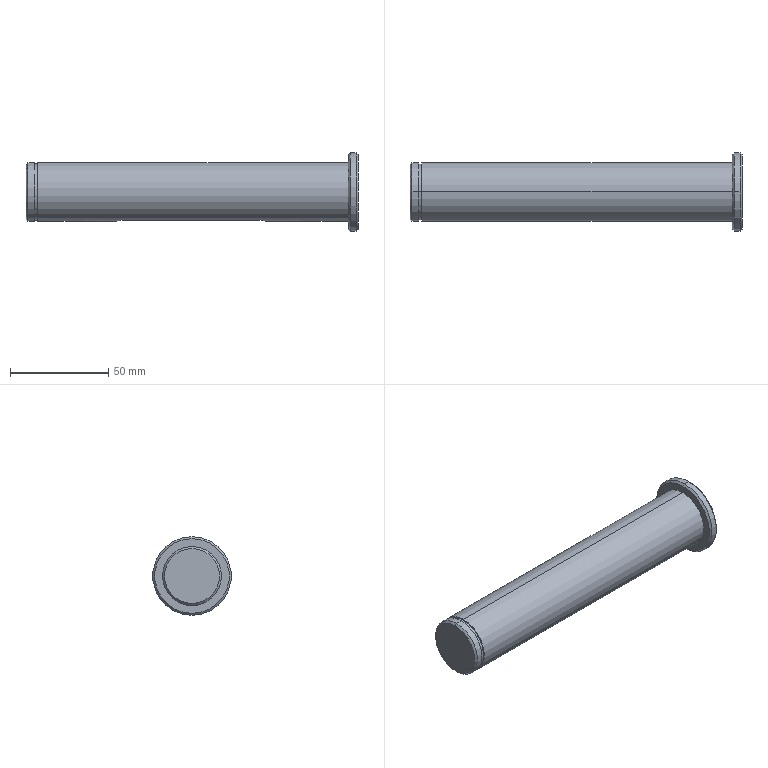Part | SolidWorks | features Chamfer 1, ICE 1, Revolution 1 | 1 solid | 25 faces | box 169 x 40 x 40 mm | volume 119602 mm3 | cylinder 11 | plane 8 | cone 6 | commonest cylinder face diameters 30 x4 8 x3 28.6 x2 40 x2
STEP:
#1=CARTESIAN_POINT('',(0.,0.,14.));
#2=VERTEX_POINT('',#1);
#3=CARTESIAN_POINT('',(0.,0.,-14.));
#4=VERTEX_POINT('',#3);
#5=CARTESIAN_POINT('',(0.,0.,0.));
#6=DIRECTION('',(-1.,0.,0.));
#7=DIRECTION('',(0.,0.,-1.));
#8=AXIS2_PLACEMENT_3D('',#5,#6,#7);
#9=CIRCLE('',#8,14.);
#10=EDGE_CURVE('',#2,#4,#9,.T.);
#11=ORIENTED_EDGE('',*,*,#10,.F.);
#12=CARTESIAN_POINT('',(1.,0.,15.));
#13=VERTEX_POINT('',#12);
#14=CARTESIAN_POINT('',(0.,0.,14.));
#15=DIRECTION('',(0.7071,0.,0.7071));
#16=VECTOR('',#15,1000.);
#17=LINE('',#14,#16);
#18=EDGE_CURVE('',#2,#13,#17,.T.);
#19=ORIENTED_EDGE('',*,*,#18,.T.);
#20=CARTESIAN_POINT('',(1.,0.,-15.));
#21=VERTEX_POINT('',#20);
#22=CARTESIAN_POINT('',(1.,0.,0.));
#23=DIRECTION('',(1.,0.,0.));
#24=DIRECTION('',(0.,0.,-1.));
#25=AXIS2_PLACEMENT_3D('',#22,#23,#24);
#26=CIRCLE('',#25,15.);
#27=EDGE_CURVE('',#21,#13,#26,.T.);
#28=ORIENTED_EDGE('',*,*,#27,.F.);
#29=CARTESIAN_POINT('',(0.,0.,-14.));
#30=DIRECTION('',(0.7071,0.,-0.7071));
#31=VECTOR('',#30,1000.);
#32=LINE('',#29,#31);
#33=EDGE_CURVE('',#4,#21,#32,.T.);
#34=ORIENTED_EDGE('',*,*,#33,.F.);
#35=EDGE_LOOP('',(#11,#19,#28,#34));
#36=FACE_OUTER_BOUND('',#35,.T.);
#37=CARTESIAN_POINT('',(0.,0.,0.));
#38=DIRECTION('',(1.,0.,0.));
#39=DIRECTION('',(0.,0.,-1.));
#40=AXIS2_PLACEMENT_3D('',#37,#38,#39);
#41=CONICAL_SURFACE('',#40,14.,0.7854);
#42=ADVANCED_FACE('',(#36),#41,.T.);
#43=CARTESIAN_POINT('',(169.,0.,-19.));
#44=VERTEX_POINT('',#43);
#45=CARTESIAN_POINT('',(169.,0.,19.));
#46=VERTEX_POINT('',#45);
#47=CARTESIAN_POINT('',(169.,0.,0.));
#48=DIRECTION('',(1.,0.,0.));
#49=DIRECTION('',(0.,0.,1.));
#50=AXIS2_PLACEMENT_3D('',#47,#48,#49);
#51=CIRCLE('',#50,19.);
#52=EDGE_CURVE('',#44,#46,#51,.T.);
#53=ORIENTED_EDGE('',*,*,#52,.F.);
#54=CARTESIAN_POINT('',(168.,0.,-20.));
#55=VERTEX_POINT('',#54);
#56=CARTESIAN_POINT('',(168.,0.,-20.));
#57=DIRECTION('',(-0.7071,0.,-0.7071));
#58=VECTOR('',#57,1000.);
#59=LINE('',#56,#58);
#60=EDGE_CURVE('',#44,#55,#59,.T.);
#61=ORIENTED_EDGE('',*,*,#60,.T.);
#62=CARTESIAN_POINT('',(168.,0.,20.));
#63=VERTEX_POINT('',#62);
#64=CARTESIAN_POINT('',(168.,0.,0.));
#65=DIRECTION('',(-1.,0.,0.));
#66=DIRECTION('',(0.,0.,1.));
#67=AXIS2_PLACEMENT_3D('',#64,#65,#66);
#68=CIRCLE('',#67,20.);
#69=EDGE_CURVE('',#63,#55,#68,.T.);
#70=ORIENTED_EDGE('',*,*,#69,.F.);
#71=CARTESIAN_POINT('',(168.,0.,20.));
#72=DIRECTION('',(-0.7071,0.,0.7071));
#73=VECTOR('',#72,1000.);
#74=LINE('',#71,#73);
#75=EDGE_CURVE('',#46,#63,#74,.T.);
#76=ORIENTED_EDGE('',*,*,#75,.F.);
#77=EDGE_LOOP('',(#53,#61,#70,#76));
#78=FACE_OUTER_BOUND('',#77,.T.);
#79=CARTESIAN_POINT('',(168.,0.,0.));
#80=DIRECTION('',(-1.,0.,0.));
#81=DIRECTION('',(0.,0.,1.));
#82=AXIS2_PLACEMENT_3D('',#79,#80,#81);
#83=CONICAL_SURFACE('',#82,20.,0.7854);
#84=ADVANCED_FACE('',(#78),#83,.T.);
#85=CARTESIAN_POINT('',(164.,0.,19.));
#86=VERTEX_POINT('',#85);
#87=CARTESIAN_POINT('',(164.,0.,-19.));
#88=VERTEX_POINT('',#87);
#89=CARTESIAN_POINT('',(164.,0.,0.));
#90=DIRECTION('',(-1.,0.,0.));
#91=DIRECTION('',(0.,0.,-1.));
#92=AXIS2_PLACEMENT_3D('',#89,#90,#91);
#93=CIRCLE('',#92,19.);
#94=EDGE_CURVE('',#86,#88,#93,.T.);
#95=ORIENTED_EDGE('',*,*,#94,.F.);
#96=CARTESIAN_POINT('',(165.,0.,20.));
#97=VERTEX_POINT('',#96);
#98=CARTESIAN_POINT('',(164.,0.,19.));
#99=DIRECTION('',(0.7071,0.,0.7071));
#100=VECTOR('',#99,1000.);
#101=LINE('',#98,#100);
#102=EDGE_CURVE('',#86,#97,#101,.T.);
#103=ORIENTED_EDGE('',*,*,#102,.T.);
#104=CARTESIAN_POINT('',(165.,0.,-20.));
#105=VERTEX_POINT('',#104);
#106=CARTESIAN_POINT('',(165.,0.,0.));
#107=DIRECTION('',(1.,0.,0.));
#108=DIRECTION('',(0.,0.,-1.));
#109=AXIS2_PLACEMENT_3D('',#106,#107,#108);
#110=CIRCLE('',#109,20.);
#111=EDGE_CURVE('',#105,#97,#110,.T.);
#112=ORIENTED_EDGE('',*,*,#111,.F.);
#113=CARTESIAN_POINT('',(164.,0.,-19.));
#114=DIRECTION('',(0.7071,0.,-0.7071));
#115=VECTOR('',#114,1000.);
#116=LINE('',#113,#115);
#117=EDGE_CURVE('',#88,#105,#116,.T.);
#118=ORIENTED_EDGE('',*,*,#117,.F.);
#119=EDGE_LOOP('',(#95,#103,#112,#118));
#120=FACE_OUTER_BOUND('',#119,.T.);
#121=CARTESIAN_POINT('',(164.,0.,0.));
#122=DIRECTION('',(1.,0.,0.));
#123=DIRECTION('',(0.,0.,-1.));
#124=AXIS2_PLACEMENT_3D('',#121,#122,#123);
#125=CONICAL_SURFACE('',#124,19.,0.7854);
#126=ADVANCED_FACE('',(#120),#125,.T.);
#127=CARTESIAN_POINT('',(49.,4.,-11.));
#128=VERTEX_POINT('',#127);
#129=CARTESIAN_POINT('',(45.,0.,-11.));
#130=VERTEX_POINT('',#129);
#131=CARTESIAN_POINT('',(49.,0.,-11.));
#132=DIRECTION('',(0.,0.,1.));
#133=DIRECTION('',(1.,0.,0.));
#134=AXIS2_PLACEMENT_3D('',#131,#132,#133);
#135=CIRCLE('',#134,4.);
#136=EDGE_CURVE('',#128,#130,#135,.T.);
#137=ORIENTED_EDGE('',*,*,#136,.T.);
#138=CARTESIAN_POINT('',(45.,0.,-15.));
#139=VERTEX_POINT('',#138);
#140=CARTESIAN_POINT('',(45.,0.,-11.));
#141=DIRECTION('',(0.,0.,-1.));
#142=VECTOR('',#141,1000.);
#143=LINE('',#140,#142);
#144=EDGE_CURVE('',#130,#139,#143,.T.);
#145=ORIENTED_EDGE('',*,*,#144,.T.);
#146=CARTESIAN_POINT('',(49.,4.,-14.457));
#147=VERTEX_POINT('',#146);
#148=CARTESIAN_POINT('',(45.,0.,-15.));
#149=CARTESIAN_POINT('',(45.,0.262,-15.));
#150=CARTESIAN_POINT('',(45.026,0.5282,-14.993));
#151=CARTESIAN_POINT('',(45.129,1.042,-14.966));
#152=CARTESIAN_POINT('',(45.205,1.292,-14.946));
#153=CARTESIAN_POINT('',(45.508,2.02,-14.871));
#154=CARTESIAN_POINT('',(45.802,2.459,-14.802));
#155=CARTESIAN_POINT('',(46.357,3.014,-14.695));
#156=CARTESIAN_POINT('',(46.557,3.178,-14.66));
#157=CARTESIAN_POINT('',(46.989,3.467,-14.594));
#158=CARTESIAN_POINT('',(47.223,3.593,-14.564));
#159=CARTESIAN_POINT('',(47.705,3.794,-14.513));
#160=CARTESIAN_POINT('',(47.954,3.87,-14.492));
#161=CARTESIAN_POINT('',(48.469,3.973,-14.464));
#162=CARTESIAN_POINT('',(48.735,4.,-14.457));
#163=CARTESIAN_POINT('',(49.,4.,-14.457));
#164=B_SPLINE_CURVE_WITH_KNOTS('',3,(#148,#149,#150,#151,#152,#153,#154,#155,#156,#157,#158,#159,#160,#161,#162,#163),.UNSPECIFIED.,.F.,.F.,(4,2,2,2,2,2,2,4),(0.006283,0.007068,0.007852,0.009421,0.01021,0.01099,0.01177,0.01256),.UNSPECIFIED.);
#165=EDGE_CURVE('',#139,#147,#164,.T.);
#166=ORIENTED_EDGE('',*,*,#165,.T.);
#167=CARTESIAN_POINT('',(49.,4.,-11.));
#168=DIRECTION('',(0.,0.,-1.));
#169=VECTOR('',#168,1000.);
#170=LINE('',#167,#169);
#171=EDGE_CURVE('',#128,#147,#170,.T.);
#172=ORIENTED_EDGE('',*,*,#171,.F.);
#173=EDGE_LOOP('',(#137,#145,#166,#172));
#174=FACE_OUTER_BOUND('',#173,.T.);
#175=CARTESIAN_POINT('',(49.,0.,-11.));
#176=DIRECTION('',(0.,0.,-1.));
#177=DIRECTION('',(-1.,0.,0.));
#178=AXIS2_PLACEMENT_3D('',#175,#176,#177);
#179=CYLINDRICAL_SURFACE('',#178,4.);
#180=ADVANCED_FACE('',(#174),#179,.F.);
#181=ORIENTED_EDGE('',*,*,#69,.T.);
#182=CARTESIAN_POINT('',(0.,0.,-20.));
#183=DIRECTION('',(-1.,0.,0.));
#184=VECTOR('',#183,1000.);
#185=LINE('',#182,#184);
#186=EDGE_CURVE('',#55,#105,#185,.T.);
#187=ORIENTED_EDGE('',*,*,#186,.T.);
#188=ORIENTED_EDGE('',*,*,#111,.T.);
#189=CARTESIAN_POINT('',(0.,0.,20.));
#190=DIRECTION('',(-1.,0.,0.));
#191=VECTOR('',#190,1000.);
#192=LINE('',#189,#191);
#193=EDGE_CURVE('',#63,#97,#192,.T.);
#194=ORIENTED_EDGE('',*,*,#193,.F.);
#195=EDGE_LOOP('',(#181,#187,#188,#194));
#196=FACE_OUTER_BOUND('',#195,.T.);
#197=CARTESIAN_POINT('',(0.,0.,0.));
#198=DIRECTION('',(-1.,0.,0.));
#199=DIRECTION('',(0.,0.,1.));
#200=AXIS2_PLACEMENT_3D('',#197,#198,#199);
#201=CYLINDRICAL_SURFACE('',#200,20.);
#202=ADVANCED_FACE('',(#196),#201,.T.);
#203=CARTESIAN_POINT('',(6.,0.,14.3));
#204=VERTEX_POINT('',#203);
#205=CARTESIAN_POINT('',(6.,0.,-14.3));
#206=VERTEX_POINT('',#205);
#207=CARTESIAN_POINT('',(6.,0.,0.));
#208=DIRECTION('',(-1.,0.,0.));
#209=DIRECTION('',(0.,0.,1.));
#210=AXIS2_PLACEMENT_3D('',#207,#208,#209);
#211=CIRCLE('',#210,14.3);
#212=EDGE_CURVE('',#204,#206,#211,.T.);
#213=ORIENTED_EDGE('',*,*,#212,.T.);
#214=CARTESIAN_POINT('',(4.4,0.,-14.3));
#215=VERTEX_POINT('',#214);
#216=CARTESIAN_POINT('',(0.,0.,-14.3));
#217=DIRECTION('',(-1.,0.,0.));
#218=VECTOR('',#217,1000.);
#219=LINE('',#216,#218);
#220=EDGE_CURVE('',#206,#215,#219,.T.);
#221=ORIENTED_EDGE('',*,*,#220,.T.);
#222=CARTESIAN_POINT('',(4.4,0.,14.3));
#223=VERTEX_POINT('',#222);
#224=CARTESIAN_POINT('',(4.4,0.,0.));
#225=DIRECTION('',(-1.,0.,0.));
#226=DIRECTION('',(0.,0.,1.));
#227=AXIS2_PLACEMENT_3D('',#224,#225,#226);
#228=CIRCLE('',#227,14.3);
#229=EDGE_CURVE('',#223,#215,#228,.T.);
#230=ORIENTED_EDGE('',*,*,#229,.F.);
#231=CARTESIAN_POINT('',(0.,0.,14.3));
#232=DIRECTION('',(-1.,0.,0.));
#233=VECTOR('',#232,1000.);
#234=LINE('',#231,#233);
#235=EDGE_CURVE('',#204,#223,#234,.T.);
#236=ORIENTED_EDGE('',*,*,#235,.F.);
#237=EDGE_LOOP('',(#213,#221,#230,#236));
#238=FACE_OUTER_BOUND('',#237,.T.);
#239=CARTESIAN_POINT('',(0.,0.,0.));
#240=DIRECTION('',(-1.,0.,0.));
#241=DIRECTION('',(0.,0.,1.));
#242=AXIS2_PLACEMENT_3D('',#239,#240,#241);
#243=CYLINDRICAL_SURFACE('',#242,14.3);
#244=ADVANCED_FACE('',(#238),#243,.T.);
#245=CARTESIAN_POINT('',(4.4,0.,15.));
#246=VERTEX_POINT('',#245);
#247=CARTESIAN_POINT('',(4.4,0.,-15.));
#248=VERTEX_POINT('',#247);
#249=CARTESIAN_POINT('',(4.4,0.,0.));
#250=DIRECTION('',(-1.,0.,0.));
#251=DIRECTION('',(0.,0.,1.));
#252=AXIS2_PLACEMENT_3D('',#249,#250,#251);
#253=CIRCLE('',#252,15.);
#254=EDGE_CURVE('',#246,#248,#253,.T.);
#255=ORIENTED_EDGE('',*,*,#254,.T.);
#256=CARTESIAN_POINT('',(0.,0.,-15.));
#257=DIRECTION('',(-1.,0.,0.));
#258=VECTOR('',#257,1000.);
#259=LINE('',#256,#258);
#260=EDGE_CURVE('',#248,#21,#259,.T.);
#261=ORIENTED_EDGE('',*,*,#260,.T.);
#262=ORIENTED_EDGE('',*,*,#27,.T.);
#263=CARTESIAN_POINT('',(0.,0.,15.));
#264=DIRECTION('',(-1.,0.,0.));
#265=VECTOR('',#264,1000.);
#266=LINE('',#263,#265);
#267=EDGE_CURVE('',#246,#13,#266,.T.);
#268=ORIENTED_EDGE('',*,*,#267,.F.);
#269=EDGE_LOOP('',(#255,#261,#262,#268));
#270=FACE_OUTER_BOUND('',#269,.T.);
#271=CARTESIAN_POINT('',(0.,0.,0.));
#272=DIRECTION('',(-1.,0.,0.));
#273=DIRECTION('',(0.,0.,1.));
#274=AXIS2_PLACEMENT_3D('',#271,#272,#273);
#275=CYLINDRICAL_SURFACE('',#274,15.);
#276=ADVANCED_FACE('',(#270),#275,.T.);
#277=CARTESIAN_POINT('',(164.,0.,15.));
#278=VERTEX_POINT('',#277);
#279=CARTESIAN_POINT('',(164.,0.,-15.));
#280=VERTEX_POINT('',#279);
#281=CARTESIAN_POINT('',(164.,0.,0.));
#282=DIRECTION('',(-1.,0.,0.));
#283=DIRECTION('',(0.,0.,1.));
#284=AXIS2_PLACEMENT_3D('',#281,#282,#283);
#285=CIRCLE('',#284,15.);
#286=EDGE_CURVE('',#278,#280,#285,.T.);
#287=ORIENTED_EDGE('',*,*,#286,.T.);
#288=CARTESIAN_POINT('',(123.,0.,-15.));
#289=VERTEX_POINT('',#288);
#290=CARTESIAN_POINT('',(0.,0.,-15.));
#291=DIRECTION('',(-1.,0.,0.));
#292=VECTOR('',#291,1000.);
#293=LINE('',#290,#292);
#294=EDGE_CURVE('',#280,#289,#293,.T.);
#295=ORIENTED_EDGE('',*,*,#294,.T.);
#296=CARTESIAN_POINT('',(119.,4.,-14.457));
#297=VERTEX_POINT('',#296);
#298=CARTESIAN_POINT('',(119.,4.,-14.457));
#299=CARTESIAN_POINT('',(119.266,4.,-14.457));
#300=CARTESIAN_POINT('',(119.527,3.974,-14.464));
#301=CARTESIAN_POINT('',(120.04,3.871,-14.492));
#302=CARTESIAN_POINT('',(120.294,3.794,-14.513));
#303=CARTESIAN_POINT('',(120.778,3.593,-14.564));
#304=CARTESIAN_POINT('',(121.008,3.47,-14.594));
#305=CARTESIAN_POINT('',(121.442,3.179,-14.66));
#306=CARTESIAN_POINT('',(121.646,3.011,-14.696));
#307=CARTESIAN_POINT('',(122.013,2.644,-14.766));
#308=CARTESIAN_POINT('',(122.178,2.443,-14.801));
#309=CARTESIAN_POINT('',(122.471,2.006,-14.867));
#310=CARTESIAN_POINT('',(122.594,1.775,-14.897));
#311=CARTESIAN_POINT('',(122.794,1.293,-14.946));
#312=CARTESIAN_POINT('',(122.871,1.04,-14.966));
#313=CARTESIAN_POINT('',(122.974,0.5228,-14.993));
#314=CARTESIAN_POINT('',(123.,0.2623,-15.));
#315=CARTESIAN_POINT('',(123.,0.,-15.));
#316=B_SPLINE_CURVE_WITH_KNOTS('',3,(#298,#299,#300,#301,#302,#303,#304,#305,#306,#307,#308,#309,#310,#311,#312,#313,#314,#315),.UNSPECIFIED.,.F.,.F.,(4,2,2,2,2,2,2,2,4),(0.,0.0007854,0.001571,0.002356,0.003142,0.003927,0.004712,0.005498,0.006283),.UNSPECIFIED.);
#317=EDGE_CURVE('',#297,#289,#316,.T.);
#318=ORIENTED_EDGE('',*,*,#317,.F.);
#319=CARTESIAN_POINT('',(0.,4.,-14.457));
#320=DIRECTION('',(1.,0.,0.));
#321=VECTOR('',#320,1000.);
#322=LINE('',#319,#321);
#323=EDGE_CURVE('',#147,#297,#322,.T.);
#324=ORIENTED_EDGE('',*,*,#323,.F.);
#325=ORIENTED_EDGE('',*,*,#165,.F.);
#326=CARTESIAN_POINT('',(6.,0.,-15.));
#327=VERTEX_POINT('',#326);
#328=CARTESIAN_POINT('',(0.,0.,-15.));
#329=DIRECTION('',(-1.,0.,0.));
#330=VECTOR('',#329,1000.);
#331=LINE('',#328,#330);
#332=EDGE_CURVE('',#139,#327,#331,.T.);
#333=ORIENTED_EDGE('',*,*,#332,.T.);
#334=CARTESIAN_POINT('',(6.,0.,15.));
#335=VERTEX_POINT('',#334);
#336=CARTESIAN_POINT('',(6.,0.,0.));
#337=DIRECTION('',(-1.,0.,0.));
#338=DIRECTION('',(0.,0.,1.));
#339=AXIS2_PLACEMENT_3D('',#336,#337,#338);
#340=CIRCLE('',#339,15.);
#341=EDGE_CURVE('',#335,#327,#340,.T.);
#342=ORIENTED_EDGE('',*,*,#341,.F.);
#343=CARTESIAN_POINT('',(0.,0.,15.));
#344=DIRECTION('',(-1.,0.,0.));
#345=VECTOR('',#344,1000.);
#346=LINE('',#343,#345);
#347=EDGE_CURVE('',#278,#335,#346,.T.);
#348=ORIENTED_EDGE('',*,*,#347,.F.);
#349=EDGE_LOOP('',(#287,#295,#318,#324,#325,#333,#342,#348));
#350=FACE_OUTER_BOUND('',#349,.T.);
#351=CARTESIAN_POINT('',(0.,0.,0.));
#352=DIRECTION('',(-1.,0.,0.));
#353=DIRECTION('',(0.,0.,1.));
#354=AXIS2_PLACEMENT_3D('',#351,#352,#353);
#355=CYLINDRICAL_SURFACE('',#354,15.);
#356=ADVANCED_FACE('',(#350),#355,.T.);
#357=ORIENTED_EDGE('',*,*,#294,.F.);
#358=CARTESIAN_POINT('',(164.,0.,0.));
#359=DIRECTION('',(-1.,0.,0.));
#360=DIRECTION('',(0.,0.,1.));
#361=AXIS2_PLACEMENT_3D('',#358,#359,#360);
#362=CIRCLE('',#361,15.);
#363=EDGE_CURVE('',#280,#278,#362,.T.);
#364=ORIENTED_EDGE('',*,*,#363,.T.);
#365=ORIENTED_EDGE('',*,*,#347,.T.);
#366=CARTESIAN_POINT('',(6.,0.,0.));
#367=DIRECTION('',(-1.,0.,0.));
#368=DIRECTION('',(0.,0.,1.));
#369=AXIS2_PLACEMENT_3D('',#366,#367,#368);
#370=CIRCLE('',#369,15.);
#371=EDGE_CURVE('',#327,#335,#370,.T.);
#372=ORIENTED_EDGE('',*,*,#371,.F.);
#373=ORIENTED_EDGE('',*,*,#332,.F.);
#374=CARTESIAN_POINT('',(49.,-4.,-14.457));
#375=VERTEX_POINT('',#374);
#376=CARTESIAN_POINT('',(49.,-4.,-14.457));
#377=CARTESIAN_POINT('',(48.734,-4.,-14.457));
#378=CARTESIAN_POINT('',(48.473,-3.974,-14.464));
#379=CARTESIAN_POINT('',(47.96,-3.871,-14.492));
#380=CARTESIAN_POINT('',(47.706,-3.794,-14.513));
#381=CARTESIAN_POINT('',(47.222,-3.593,-14.564));
#382=CARTESIAN_POINT('',(46.992,-3.47,-14.594));
#383=CARTESIAN_POINT('',(46.558,-3.179,-14.66));
#384=CARTESIAN_POINT('',(46.354,-3.011,-14.696));
#385=CARTESIAN_POINT('',(45.987,-2.644,-14.766));
#386=CARTESIAN_POINT('',(45.822,-2.443,-14.801));
#387=CARTESIAN_POINT('',(45.529,-2.006,-14.867));
#388=CARTESIAN_POINT('',(45.406,-1.775,-14.897));
#389=CARTESIAN_POINT('',(45.206,-1.293,-14.946));
#390=CARTESIAN_POINT('',(45.129,-1.04,-14.966));
#391=CARTESIAN_POINT('',(45.026,-0.5228,-14.993));
#392=CARTESIAN_POINT('',(45.,-0.2623,-15.));
#393=CARTESIAN_POINT('',(45.,0.,-15.));
#394=B_SPLINE_CURVE_WITH_KNOTS('',3,(#376,#377,#378,#379,#380,#381,#382,#383,#384,#385,#386,#387,#388,#389,#390,#391,#392,#393),.UNSPECIFIED.,.F.,.F.,(4,2,2,2,2,2,2,2,4),(0.,0.0007854,0.001571,0.002356,0.003142,0.003927,0.004712,0.005498,0.006283),.UNSPECIFIED.);
#395=EDGE_CURVE('',#375,#139,#394,.T.);
#396=ORIENTED_EDGE('',*,*,#395,.F.);
#397=CARTESIAN_POINT('',(119.,-4.,-14.457));
#398=VERTEX_POINT('',#397);
#399=CARTESIAN_POINT('',(0.,-4.,-14.457));
#400=DIRECTION('',(-1.,0.,0.));
#401=VECTOR('',#400,1000.);
#402=LINE('',#399,#401);
#403=EDGE_CURVE('',#398,#375,#402,.T.);
#404=ORIENTED_EDGE('',*,*,#403,.F.);
#405=CARTESIAN_POINT('',(123.,0.,-15.));
#406=CARTESIAN_POINT('',(123.,-0.262,-15.));
#407=CARTESIAN_POINT('',(122.974,-0.5282,-14.993));
#408=CARTESIAN_POINT('',(122.871,-1.042,-14.966));
#409=CARTESIAN_POINT('',(122.795,-1.292,-14.946));
#410=CARTESIAN_POINT('',(122.492,-2.02,-14.871));
#411=CARTESIAN_POINT('',(122.198,-2.459,-14.802));
#412=CARTESIAN_POINT('',(121.643,-3.014,-14.695));
#413=CARTESIAN_POINT('',(121.443,-3.178,-14.66));
#414=CARTESIAN_POINT('',(121.011,-3.467,-14.594));
#415=CARTESIAN_POINT('',(120.777,-3.593,-14.564));
#416=CARTESIAN_POINT('',(120.295,-3.794,-14.513));
#417=CARTESIAN_POINT('',(120.046,-3.87,-14.492));
#418=CARTESIAN_POINT('',(119.531,-3.973,-14.464));
#419=CARTESIAN_POINT('',(119.265,-4.,-14.457));
#420=CARTESIAN_POINT('',(119.,-4.,-14.457));
#421=B_SPLINE_CURVE_WITH_KNOTS('',3,(#405,#406,#407,#408,#409,#410,#411,#412,#413,#414,#415,#416,#417,#418,#419,#420),.UNSPECIFIED.,.F.,.F.,(4,2,2,2,2,2,2,4),(0.006283,0.007068,0.007852,0.009421,0.01021,0.01099,0.01177,0.01256),.UNSPECIFIED.);
#422=EDGE_CURVE('',#289,#398,#421,.T.);
#423=ORIENTED_EDGE('',*,*,#422,.F.);
#424=EDGE_LOOP('',(#357,#364,#365,#372,#373,#396,#404,#423));
#425=FACE_OUTER_BOUND('',#424,.T.);
#426=CARTESIAN_POINT('',(0.,0.,0.));
#427=DIRECTION('',(-1.,0.,0.));
#428=DIRECTION('',(0.,0.,1.));
#429=AXIS2_PLACEMENT_3D('',#426,#427,#428);
#430=CYLINDRICAL_SURFACE('',#429,15.);
#431=ADVANCED_FACE('',(#425),#430,.T.);
#432=CARTESIAN_POINT('',(0.,0.,0.));
#433=DIRECTION('',(-1.,0.,0.));
#434=DIRECTION('',(0.,0.,-1.));
#435=AXIS2_PLACEMENT_3D('',#432,#433,#434);
#436=CIRCLE('',#435,14.);
#437=EDGE_CURVE('',#4,#2,#436,.T.);
#438=ORIENTED_EDGE('',*,*,#437,.T.);
#439=ORIENTED_EDGE('',*,*,#10,.T.);
#440=EDGE_LOOP('',(#438,#439));
#441=FACE_OUTER_BOUND('',#440,.T.);
#442=CARTESIAN_POINT('',(0.,0.,0.));
#443=DIRECTION('',(1.,0.,0.));
#444=DIRECTION('',(0.,0.,-1.));
#445=AXIS2_PLACEMENT_3D('',#442,#443,#444);
#446=PLANE('',#445);
#447=ADVANCED_FACE('',(#441),#446,.F.);
#448=ORIENTED_EDGE('',*,*,#260,.F.);
#449=CARTESIAN_POINT('',(4.4,0.,0.));
#450=DIRECTION('',(-1.,0.,0.));
#451=DIRECTION('',(0.,0.,1.));
#452=AXIS2_PLACEMENT_3D('',#449,#450,#451);
#453=CIRCLE('',#452,15.);
#454=EDGE_CURVE('',#248,#246,#453,.T.);
#455=ORIENTED_EDGE('',*,*,#454,.T.);
#456=ORIENTED_EDGE('',*,*,#267,.T.);
#457=CARTESIAN_POINT('',(1.,0.,0.));
#458=DIRECTION('',(1.,0.,0.));
#459=DIRECTION('',(0.,0.,-1.));
#460=AXIS2_PLACEMENT_3D('',#457,#458,#459);
#461=CIRCLE('',#460,15.);
#462=EDGE_CURVE('',#13,#21,#461,.T.);
#463=ORIENTED_EDGE('',*,*,#462,.T.);
#464=EDGE_LOOP('',(#448,#455,#456,#463));
#465=FACE_OUTER_BOUND('',#464,.T.);
#466=CARTESIAN_POINT('',(0.,0.,0.));
#467=DIRECTION('',(-1.,0.,0.));
#468=DIRECTION('',(0.,0.,1.));
#469=AXIS2_PLACEMENT_3D('',#466,#467,#468);
#470=CYLINDRICAL_SURFACE('',#469,15.);
#471=ADVANCED_FACE('',(#465),#470,.T.);
#472=ORIENTED_EDGE('',*,*,#254,.F.);
#473=ORIENTED_EDGE('',*,*,#454,.F.);
#474=EDGE_LOOP('',(#472,#473));
#475=FACE_OUTER_BOUND('',#474,.T.);
#476=ORIENTED_EDGE('',*,*,#229,.T.);
#477=CARTESIAN_POINT('',(4.4,0.,0.));
#478=DIRECTION('',(-1.,0.,0.));
#479=DIRECTION('',(0.,0.,1.));
#480=AXIS2_PLACEMENT_3D('',#477,#478,#479);
#481=CIRCLE('',#480,14.3);
#482=EDGE_CURVE('',#215,#223,#481,.T.);
#483=ORIENTED_EDGE('',*,*,#482,.T.);
#484=EDGE_LOOP('',(#476,#483));
#485=FACE_BOUND('',#484,.T.);
#486=CARTESIAN_POINT('',(4.4,15.,0.));
#487=DIRECTION('',(-1.,0.,0.));
#488=DIRECTION('',(0.,0.,1.));
#489=AXIS2_PLACEMENT_3D('',#486,#487,#488);
#490=PLANE('',#489);
#491=ADVANCED_FACE('',(#475,#485),#490,.F.);
#492=ORIENTED_EDGE('',*,*,#220,.F.);
#493=CARTESIAN_POINT('',(6.,0.,0.));
#494=DIRECTION('',(-1.,0.,0.));
#495=DIRECTION('',(0.,0.,1.));
#496=AXIS2_PLACEMENT_3D('',#493,#494,#495);
#497=CIRCLE('',#496,14.3);
#498=EDGE_CURVE('',#206,#204,#497,.T.);
#499=ORIENTED_EDGE('',*,*,#498,.T.);
#500=ORIENTED_EDGE('',*,*,#235,.T.);
#501=ORIENTED_EDGE('',*,*,#482,.F.);
#502=EDGE_LOOP('',(#492,#499,#500,#501));
#503=FACE_OUTER_BOUND('',#502,.T.);
#504=CARTESIAN_POINT('',(0.,0.,0.));
#505=DIRECTION('',(-1.,0.,0.));
#506=DIRECTION('',(0.,0.,1.));
#507=AXIS2_PLACEMENT_3D('',#504,#505,#506);
#508=CYLINDRICAL_SURFACE('',#507,14.3);
#509=ADVANCED_FACE('',(#503),#508,.T.);
#510=ORIENTED_EDGE('',*,*,#212,.F.);
#511=ORIENTED_EDGE('',*,*,#498,.F.);
#512=EDGE_LOOP('',(#510,#511));
#513=FACE_BOUND('',#512,.T.);
#514=ORIENTED_EDGE('',*,*,#341,.T.);
#515=ORIENTED_EDGE('',*,*,#371,.T.);
#516=EDGE_LOOP('',(#514,#515));
#517=FACE_OUTER_BOUND('',#516,.T.);
#518=CARTESIAN_POINT('',(6.,14.3,0.));
#519=DIRECTION('',(1.,0.,0.));
#520=DIRECTION('',(0.,0.,-1.));
#521=AXIS2_PLACEMENT_3D('',#518,#519,#520);
#522=PLANE('',#521);
#523=ADVANCED_FACE('',(#513,#517),#522,.F.);
#524=CARTESIAN_POINT('',(164.,0.,0.));
#525=DIRECTION('',(-1.,0.,0.));
#526=DIRECTION('',(0.,0.,-1.));
#527=AXIS2_PLACEMENT_3D('',#524,#525,#526);
#528=CIRCLE('',#527,19.);
#529=EDGE_CURVE('',#88,#86,#528,.T.);
#530=ORIENTED_EDGE('',*,*,#529,.T.);
#531=ORIENTED_EDGE('',*,*,#94,.T.);
#532=EDGE_LOOP('',(#530,#531));
#533=FACE_OUTER_BOUND('',#532,.T.);
#534=ORIENTED_EDGE('',*,*,#286,.F.);
#535=ORIENTED_EDGE('',*,*,#363,.F.);
#536=EDGE_LOOP('',(#534,#535));
#537=FACE_BOUND('',#536,.T.);
#538=CARTESIAN_POINT('',(164.,15.,0.));
#539=DIRECTION('',(1.,0.,0.));
#540=DIRECTION('',(0.,0.,-1.));
#541=AXIS2_PLACEMENT_3D('',#538,#539,#540);
#542=PLANE('',#541);
#543=ADVANCED_FACE('',(#533,#537),#542,.F.);
#544=ORIENTED_EDGE('',*,*,#186,.F.);
#545=CARTESIAN_POINT('',(168.,0.,0.));
#546=DIRECTION('',(-1.,0.,0.));
#547=DIRECTION('',(0.,0.,1.));
#548=AXIS2_PLACEMENT_3D('',#545,#546,#547);
#549=CIRCLE('',#548,20.);
#550=EDGE_CURVE('',#55,#63,#549,.T.);
#551=ORIENTED_EDGE('',*,*,#550,.T.);
#552=ORIENTED_EDGE('',*,*,#193,.T.);
#553=CARTESIAN_POINT('',(165.,0.,0.));
#554=DIRECTION('',(1.,0.,0.));
#555=DIRECTION('',(0.,0.,-1.));
#556=AXIS2_PLACEMENT_3D('',#553,#554,#555);
#557=CIRCLE('',#556,20.);
#558=EDGE_CURVE('',#97,#105,#557,.T.);
#559=ORIENTED_EDGE('',*,*,#558,.T.);
#560=EDGE_LOOP('',(#544,#551,#552,#559));
#561=FACE_OUTER_BOUND('',#560,.T.);
#562=CARTESIAN_POINT('',(0.,0.,0.));
#563=DIRECTION('',(-1.,0.,0.));
#564=DIRECTION('',(0.,0.,1.));
#565=AXIS2_PLACEMENT_3D('',#562,#563,#564);
#566=CYLINDRICAL_SURFACE('',#565,20.);
#567=ADVANCED_FACE('',(#561),#566,.T.);
#568=CARTESIAN_POINT('',(169.,0.,0.));
#569=DIRECTION('',(1.,0.,0.));
#570=DIRECTION('',(0.,0.,1.));
#571=AXIS2_PLACEMENT_3D('',#568,#569,#570);
#572=CIRCLE('',#571,19.);
#573=EDGE_CURVE('',#46,#44,#572,.T.);
#574=ORIENTED_EDGE('',*,*,#573,.T.);
#575=ORIENTED_EDGE('',*,*,#52,.T.);
#576=EDGE_LOOP('',(#574,#575));
#577=FACE_OUTER_BOUND('',#576,.T.);
#578=CARTESIAN_POINT('',(169.,20.,0.));
#579=DIRECTION('',(-1.,0.,0.));
#580=DIRECTION('',(0.,0.,1.));
#581=AXIS2_PLACEMENT_3D('',#578,#579,#580);
#582=PLANE('',#581);
#583=ADVANCED_FACE('',(#577),#582,.F.);
#584=CARTESIAN_POINT('',(119.,4.,-11.));
#585=VERTEX_POINT('',#584);
#586=CARTESIAN_POINT('',(119.,4.,-11.));
#587=DIRECTION('',(0.,0.,-1.));
#588=VECTOR('',#587,1000.);
#589=LINE('',#586,#588);
#590=EDGE_CURVE('',#585,#297,#589,.T.);
#591=ORIENTED_EDGE('',*,*,#590,.T.);
#592=ORIENTED_EDGE('',*,*,#317,.T.);
#593=ORIENTED_EDGE('',*,*,#422,.T.);
#594=CARTESIAN_POINT('',(119.,-4.,-11.));
#595=VERTEX_POINT('',#594);
#596=CARTESIAN_POINT('',(119.,-4.,-11.));
#597=DIRECTION('',(0.,0.,-1.));
#598=VECTOR('',#597,1000.);
#599=LINE('',#596,#598);
#600=EDGE_CURVE('',#595,#398,#599,.T.);
#601=ORIENTED_EDGE('',*,*,#600,.F.);
#602=CARTESIAN_POINT('',(119.,0.,-11.));
#603=DIRECTION('',(0.,0.,1.));
#604=DIRECTION('',(1.,0.,0.));
#605=AXIS2_PLACEMENT_3D('',#602,#603,#604);
#606=CIRCLE('',#605,4.);
#607=EDGE_CURVE('',#595,#585,#606,.T.);
#608=ORIENTED_EDGE('',*,*,#607,.T.);
#609=EDGE_LOOP('',(#591,#592,#593,#601,#608));
#610=FACE_OUTER_BOUND('',#609,.T.);
#611=CARTESIAN_POINT('',(119.,0.,-11.));
#612=DIRECTION('',(0.,0.,-1.));
#613=DIRECTION('',(-1.,0.,0.));
#614=AXIS2_PLACEMENT_3D('',#611,#612,#613);
#615=CYLINDRICAL_SURFACE('',#614,4.);
#616=ADVANCED_FACE('',(#610),#615,.F.);
#617=ORIENTED_EDGE('',*,*,#323,.T.);
#618=ORIENTED_EDGE('',*,*,#590,.F.);
#619=CARTESIAN_POINT('',(119.,4.,-11.));
#620=DIRECTION('',(-1.,0.,0.));
#621=VECTOR('',#620,1000.);
#622=LINE('',#619,#621);
#623=EDGE_CURVE('',#585,#128,#622,.T.);
#624=ORIENTED_EDGE('',*,*,#623,.T.);
#625=ORIENTED_EDGE('',*,*,#171,.T.);
#626=EDGE_LOOP('',(#617,#618,#624,#625));
#627=FACE_OUTER_BOUND('',#626,.T.);
#628=CARTESIAN_POINT('',(119.,4.,-11.));
#629=DIRECTION('',(0.,-1.,0.));
#630=DIRECTION('',(1.,0.,0.));
#631=AXIS2_PLACEMENT_3D('',#628,#629,#630);
#632=PLANE('',#631);
#633=ADVANCED_FACE('',(#627),#632,.T.);
#634=ORIENTED_EDGE('',*,*,#144,.F.);
#635=CARTESIAN_POINT('',(49.,-4.,-11.));
#636=VERTEX_POINT('',#635);
#637=CARTESIAN_POINT('',(49.,0.,-11.));
#638=DIRECTION('',(0.,0.,1.));
#639=DIRECTION('',(1.,0.,0.));
#640=AXIS2_PLACEMENT_3D('',#637,#638,#639);
#641=CIRCLE('',#640,4.);
#642=EDGE_CURVE('',#130,#636,#641,.T.);
#643=ORIENTED_EDGE('',*,*,#642,.T.);
#644=CARTESIAN_POINT('',(49.,-4.,-11.));
#645=DIRECTION('',(0.,0.,-1.));
#646=VECTOR('',#645,1000.);
#647=LINE('',#644,#646);
#648=EDGE_CURVE('',#636,#375,#647,.T.);
#649=ORIENTED_EDGE('',*,*,#648,.T.);
#650=ORIENTED_EDGE('',*,*,#395,.T.);
#651=EDGE_LOOP('',(#634,#643,#649,#650));
#652=FACE_OUTER_BOUND('',#651,.T.);
#653=CARTESIAN_POINT('',(49.,0.,-11.));
#654=DIRECTION('',(0.,0.,-1.));
#655=DIRECTION('',(-1.,0.,0.));
#656=AXIS2_PLACEMENT_3D('',#653,#654,#655);
#657=CYLINDRICAL_SURFACE('',#656,4.);
#658=ADVANCED_FACE('',(#652),#657,.F.);
#659=ORIENTED_EDGE('',*,*,#403,.T.);
#660=ORIENTED_EDGE('',*,*,#648,.F.);
#661=CARTESIAN_POINT('',(119.,-4.,-11.));
#662=DIRECTION('',(1.,0.,0.));
#663=VECTOR('',#662,1000.);
#664=LINE('',#661,#663);
#665=EDGE_CURVE('',#636,#595,#664,.T.);
#666=ORIENTED_EDGE('',*,*,#665,.T.);
#667=ORIENTED_EDGE('',*,*,#600,.T.);
#668=EDGE_LOOP('',(#659,#660,#666,#667));
#669=FACE_OUTER_BOUND('',#668,.T.);
#670=CARTESIAN_POINT('',(119.,-4.,-11.));
#671=DIRECTION('',(0.,1.,0.));
#672=DIRECTION('',(-1.,0.,0.));
#673=AXIS2_PLACEMENT_3D('',#670,#671,#672);
#674=PLANE('',#673);
#675=ADVANCED_FACE('',(#669),#674,.T.);
#676=ORIENTED_EDGE('',*,*,#607,.F.);
#677=ORIENTED_EDGE('',*,*,#665,.F.);
#678=ORIENTED_EDGE('',*,*,#642,.F.);
#679=ORIENTED_EDGE('',*,*,#136,.F.);
#680=ORIENTED_EDGE('',*,*,#623,.F.);
#681=EDGE_LOOP('',(#676,#677,#678,#679,#680));
#682=FACE_OUTER_BOUND('',#681,.T.);
#683=CARTESIAN_POINT('',(119.,0.,-11.));
#684=DIRECTION('',(0.,0.,1.));
#685=DIRECTION('',(1.,0.,0.));
#686=AXIS2_PLACEMENT_3D('',#683,#684,#685);
#687=PLANE('',#686);
#688=ADVANCED_FACE('',(#682),#687,.F.);
#689=ORIENTED_EDGE('',*,*,#102,.F.);
#690=ORIENTED_EDGE('',*,*,#529,.F.);
#691=ORIENTED_EDGE('',*,*,#117,.T.);
#692=ORIENTED_EDGE('',*,*,#558,.F.);
#693=EDGE_LOOP('',(#689,#690,#691,#692));
#694=FACE_OUTER_BOUND('',#693,.T.);
#695=CARTESIAN_POINT('',(164.,0.,0.));
#696=DIRECTION('',(1.,0.,0.));
#697=DIRECTION('',(0.,0.,-1.));
#698=AXIS2_PLACEMENT_3D('',#695,#696,#697);
#699=CONICAL_SURFACE('',#698,19.,0.7854);
#700=ADVANCED_FACE('',(#694),#699,.T.);
#701=ORIENTED_EDGE('',*,*,#60,.F.);
#702=ORIENTED_EDGE('',*,*,#573,.F.);
#703=ORIENTED_EDGE('',*,*,#75,.T.);
#704=ORIENTED_EDGE('',*,*,#550,.F.);
#705=EDGE_LOOP('',(#701,#702,#703,#704));
#706=FACE_OUTER_BOUND('',#705,.T.);
#707=CARTESIAN_POINT('',(168.,0.,0.));
#708=DIRECTION('',(-1.,0.,0.));
#709=DIRECTION('',(0.,0.,1.));
#710=AXIS2_PLACEMENT_3D('',#707,#708,#709);
#711=CONICAL_SURFACE('',#710,20.,0.7854);
#712=ADVANCED_FACE('',(#706),#711,.T.);
#713=ORIENTED_EDGE('',*,*,#18,.F.);
#714=ORIENTED_EDGE('',*,*,#437,.F.);
#715=ORIENTED_EDGE('',*,*,#33,.T.);
#716=ORIENTED_EDGE('',*,*,#462,.F.);
#717=EDGE_LOOP('',(#713,#714,#715,#716));
#718=FACE_OUTER_BOUND('',#717,.T.);
#719=CARTESIAN_POINT('',(0.,0.,0.));
#720=DIRECTION('',(1.,0.,0.));
#721=DIRECTION('',(0.,0.,-1.));
#722=AXIS2_PLACEMENT_3D('',#719,#720,#721);
#723=CONICAL_SURFACE('',#722,14.,0.7854);
#724=ADVANCED_FACE('',(#718),#723,.T.);
#725=CLOSED_SHELL('',(#42,#84,#126,#180,#202,#244,#276,#356,#431,#447,#471,#491,#509,#523,#543,#567,#583,#616,#633,#658,#675,#688,#700,#712,#724));
#726=MANIFOLD_SOLID_BREP('',#725);
#727=CARTESIAN_POINT('',(0.,0.,0.));
#728=DIRECTION('',(0.,0.,1.));
#729=DIRECTION('',(1.,0.,0.));
#730=AXIS2_PLACEMENT_3D('',#727,#728,#729);
#731=(LENGTH_UNIT()NAMED_UNIT(*)SI_UNIT(.MILLI.,.METRE.));
#732=UNCERTAINTY_MEASURE_WITH_UNIT(LENGTH_MEASURE(0.00001),#731,'','');
#733=(NAMED_UNIT(*)PLANE_ANGLE_UNIT()SI_UNIT($,.RADIAN.));
#734=(NAMED_UNIT(*)SI_UNIT($,.STERADIAN.)SOLID_ANGLE_UNIT());
#735=(GEOMETRIC_REPRESENTATION_CONTEXT(3)GLOBAL_UNCERTAINTY_ASSIGNED_CONTEXT((#732))GLOBAL_UNIT_ASSIGNED_CONTEXT((#731,#733,#734))REPRESENTATION_CONTEXT('',''));
#736=ADVANCED_BREP_SHAPE_REPRESENTATION('',(#726,#730),#735);